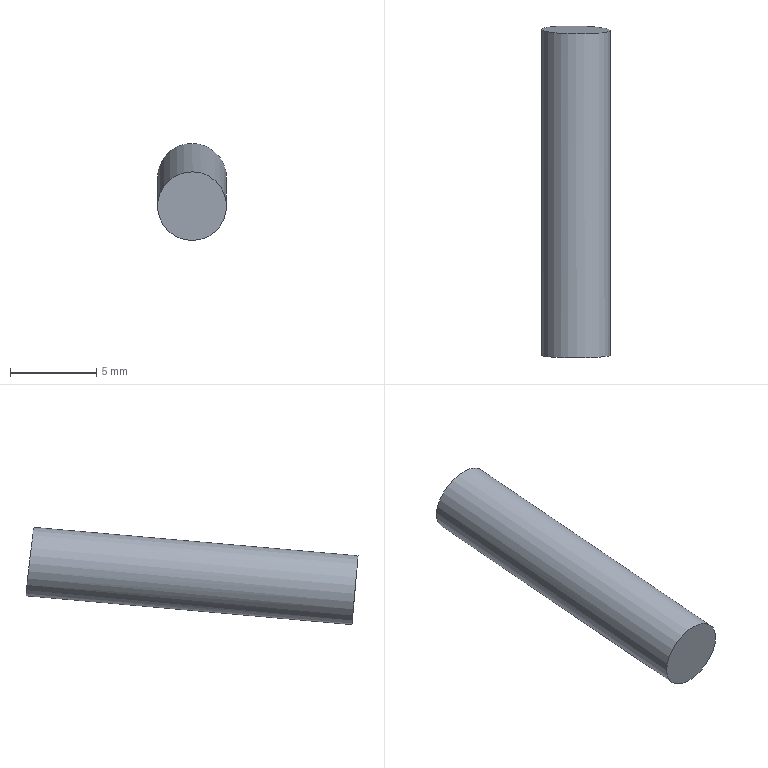Part | NX | features solid 2 | 1 solid | 3 faces | box 4 x 19.246 x 5.628 mm | volume 237.628 mm3 | plane 2 | cylinder 1 | commonest cylinder face diameters 4 x1
STEP:
#1=CARTESIAN_POINT('',(143.843,39.804,-43.998));
#2=VERTEX_POINT('',#1);
#3=CARTESIAN_POINT('',(143.325,39.972,-45.922));
#4=DIRECTION('',(0.,-0.9962,-0.08716));
#5=DIRECTION('',(0.2588,-0.08419,0.9623));
#6=AXIS2_PLACEMENT_3D('',#3,#4,#5);
#7=CIRCLE('',#6,2.);
#8=EDGE_CURVE('',#2,#2,#7,.T.);
#9=ORIENTED_EDGE('',*,*,#8,.T.);
#10=EDGE_LOOP('',(#9));
#11=FACE_BOUND('',#10,.T.);
#12=CARTESIAN_POINT('',(143.325,39.972,-45.922));
#13=DIRECTION('',(0.,-0.9962,-0.08716));
#14=DIRECTION('',(-0.2588,0.08419,-0.9623));
#15=AXIS2_PLACEMENT_3D('',#12,#13,#14);
#16=PLANE('',#15);
#17=ADVANCED_FACE('',(#11),#16,.T.);
#18=CARTESIAN_POINT('',(144.266,58.591,-42.522));
#19=VERTEX_POINT('',#18);
#20=CARTESIAN_POINT('',(143.325,58.81,-44.274));
#21=DIRECTION('',(0.01549,0.9931,0.116));
#22=DIRECTION('',(0.4705,-0.1096,0.8755));
#23=AXIS2_PLACEMENT_3D('',#20,#21,#22);
#24=ELLIPSE('',#23,2.001,2.);
#25=EDGE_CURVE('',#19,#19,#24,.T.);
#26=ORIENTED_EDGE('',*,*,#25,.T.);
#27=EDGE_LOOP('',(#26));
#28=FACE_BOUND('',#27,.T.);
#29=CARTESIAN_POINT('',(159.246,62.921,-81.584));
#30=DIRECTION('',(0.01549,0.9931,0.116));
#31=DIRECTION('',(0.06594,-0.1168,0.991));
#32=AXIS2_PLACEMENT_3D('',#29,#30,#31);
#33=PLANE('',#32);
#34=ADVANCED_FACE('',(#28),#33,.T.);
#35=ORIENTED_EDGE('',*,*,#8,.F.);
#36=EDGE_LOOP('',(#35));
#37=FACE_BOUND('',#36,.T.);
#38=ORIENTED_EDGE('',*,*,#25,.F.);
#39=EDGE_LOOP('',(#38));
#40=FACE_BOUND('',#39,.T.);
#41=CARTESIAN_POINT('',(143.325,59.896,-44.179));
#42=DIRECTION('',(0.,-0.9962,-0.08716));
#43=DIRECTION('',(-0.2588,0.08419,-0.9623));
#44=AXIS2_PLACEMENT_3D('',#41,#42,#43);
#45=CYLINDRICAL_SURFACE('',#44,2.);
#46=ADVANCED_FACE('',(#37,#40),#45,.T.);
#47=CLOSED_SHELL('',(#17,#34,#46));
#48=MANIFOLD_SOLID_BREP('',#47);
#49=(LENGTH_UNIT()NAMED_UNIT(*)SI_UNIT(.MILLI.,.METRE.));
#50=UNCERTAINTY_MEASURE_WITH_UNIT(LENGTH_MEASURE(0.00001),#49,'','');
#51=(NAMED_UNIT(*)PLANE_ANGLE_UNIT()SI_UNIT($,.RADIAN.));
#52=(NAMED_UNIT(*)SI_UNIT($,.STERADIAN.)SOLID_ANGLE_UNIT());
#53=(GEOMETRIC_REPRESENTATION_CONTEXT(3)GLOBAL_UNCERTAINTY_ASSIGNED_CONTEXT((#50))GLOBAL_UNIT_ASSIGNED_CONTEXT((#49,#51,#52))REPRESENTATION_CONTEXT('',''));
#54=ADVANCED_BREP_SHAPE_REPRESENTATION('',(#48),#53);